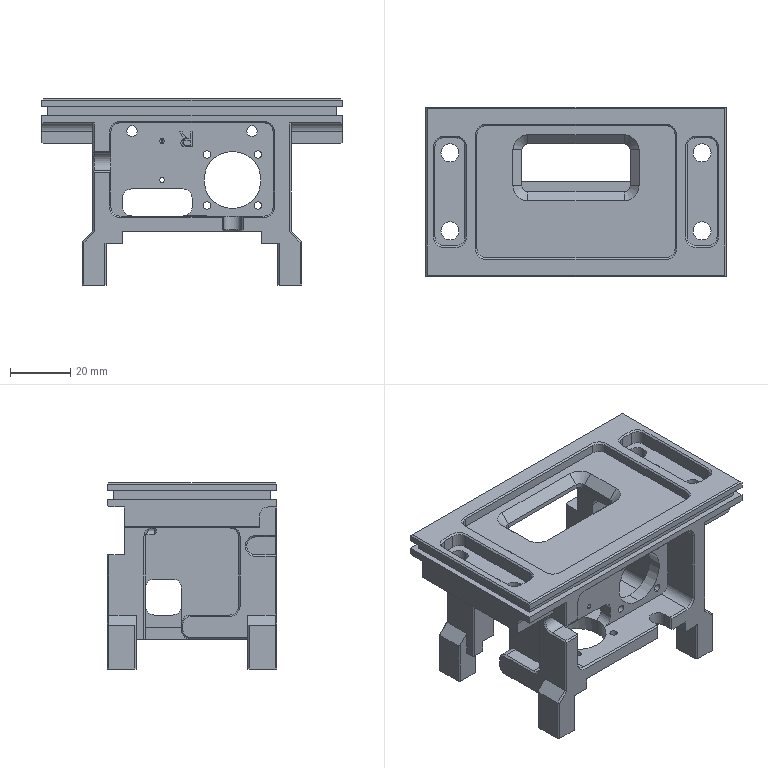NC program | Mastercam | posted with a generic post | part box 100 x 56.5 x 62 mm
Lines 30393 to 32423 of 45570, first 1872 of 2031 lines:
N6850 T11 M6
N6860 G0 G90 G17 G54 X-60. Y-16.9 A0. S8000 M3
N6870 G43 H11 Z20. M8
N6880 Z1.
N6890 G1 Z-.628 F600.
N6900 X-50. F4000.
N6910 X50.
N6920 X60.
N6930 Z-1.256 F600.
N6940 X50. F4000.
N6950 X-50.
N6960 X-60.
N6970 Z-1.883 F600.
N6980 X-50. F4000.
N6990 X50.
N7000 X60.
N7010 Z-2.511 F600.
N7020 X50. F4000.
N7030 X-50.
N7040 X-60.
N7050 Z-3.139 F600.
N7060 X-50. F4000.
N7070 X50.
N7080 X60.
N7090 Z-3.767 F600.
N7100 X50. F4000.
N7110 X-50.
N7120 X-60.
N7130 Z-4.394 F600.
N7140 X-50. F4000.
N7150 X50.
N7160 X60.
N7170 Z-5.022 F600.
N7180 X50. F4000.
N7190 X-50.
N7200 X-60.
N7210 Z-5.65 F600.
N7220 X-50. F4000.
N7230 X50.
N7240 X60.
N7250 G0 Z20.
N7260 Y-13.1
N7270 Z1.
N7280 G1 Z-.628 F600.
N7290 X50. F4000.
N7300 X-50.
N7310 X-60.
N7320 Z-1.256 F600.
N7330 X-50. F4000.
N7340 X50.
N7350 X60.
N7360 Z-1.883 F600.
N7370 X50. F4000.
N7380 X-50.
N7390 X-60.
N7400 Z-2.511 F600.
N7410 X-50. F4000.
N7420 X50.
N7430 X60.
N7440 Z-3.139 F600.
N7450 X50. F4000.
N7460 X-50.
N7470 X-60.
N7480 Z-3.767 F600.
N7490 X-50. F4000.
N7500 X50.
N7510 X60.
N7520 Z-4.394 F600.
N7530 X50. F4000.
N7540 X-50.
N7550 X-60.
N7560 Z-5.022 F600.
N7570 X-50. F4000.
N7580 X50.
N7590 X60.
N7600 Z-5.65 F600.
N7610 X50. F4000.
N7620 X-50.
N7630 X-60.
N7640 G0 Z20.
N7650 M5
N7660 G91 G28 Z0. M9
N7670 A0.
N7680 M01
N7690 T12 M6
N7700 G0 G90 G17 G54 X-60. Y-17. A0. S8000 M3
N7710 G43 H12 Z20. M8
N7720 Z-4.75
N7730 G1 Z-5.75 F600.
N7740 X-50. F1000.
N7750 X50.
N7760 X60.
N7770 G0 Z20.
N7780 Y-13.
N7790 Z-4.75
N7800 G1 Z-5.75 F600.
N7810 X50. F1000.
N7820 X-50.
N7830 X-60.
N7840 G0 Z20.
N7850 M5
N7860 G91 G28 Z0. M9
N7870 A0.
N7880 M01
N7890 T11 M6
N7900 G0 G90 G17 G54 X-2.228 Y-1.165 A0. S8000 M3
N7910 G43 H11 Z20. M8
N7920 Z1.
N7930 G1 Z.325 F600.
N7940 G3 X-7.628 Y-6.565 Z.073 I0. J-5.4 F4000.
N7950 X-2.228 Y-11.965 Z-.18 I5.4 J0.
N7960 X3.172 Y-6.565 Z-.432 I0. J5.4
N7970 X-2.228 Y-1.165 Z-.685 I-5.4 J0.
N7980 G1 X-3.035
N7990 Y-2.835
N8000 X0.
N8010 X3.035
N8020 Y-1.165
N8030 X-2.228
N8040 G2 X-2.953 Y-.582 I0. J.743
N8050 G1 X-3.73 Y2.941
N8060 G3 X-4.455 Y3.523 I-.725 J-.16
N8070 G1 X-7.723
N8080 Y-7.523
N8090 X0.
N8100 X7.723
N8110 Y3.523
N8120 X-4.455
N8130 G2 X-5.18 Y4.106 I0. J.743
N8140 G1 X-5.957 Y7.629
N8150 G3 X-6.683 Y8.212 I-.726 J-.16
N8160 G1 X-12.412
N8170 Y-12.212
N8180 X0.
N8190 X12.412
N8200 Y8.212
N8210 X-6.683
N8220 G2 X-7.408 Y8.794 I0. J.742
N8230 G1 X-8.185 Y12.317
N8240 G3 X-8.91 Y12.9 I-.725 J-.159
N8250 G1 X-16.188
N8260 X-17.087 Y12.887
N8270 X-17.1 Y12.656
N8280 Y-16.898
N8290 X-17.099 Y-16.9
N8300 X0.
N8310 X17.099
N8320 X17.1 Y12.656
N8330 X17.087 Y12.887
N8340 X16.959 Y12.898
N8350 X16.188 Y12.9
N8360 X-8.91
N8370 G0 Z20.
N8380 X-2.228 Y-1.165
N8390 Z.315
N8400 G1 Z-.36 F600.
N8410 G3 X-7.628 Y-6.565 Z-.612 I0. J-5.4 F4000.
N8420 X-2.228 Y-11.965 Z-.865 I5.4 J0.
N8430 X3.172 Y-6.565 Z-1.117 I0. J5.4
N8440 X-2.228 Y-1.165 Z-1.369 I-5.4 J0.
N8450 G1 X-3.035
N8460 Y-2.835
N8470 X0.
N8480 X3.035
N8490 Y-1.165
N8500 X-2.228
N8510 G2 X-2.953 Y-.582 I0. J.743
N8520 G1 X-3.73 Y2.941
N8530 G3 X-4.455 Y3.523 I-.725 J-.16
N8540 G1 X-7.723
N8550 Y-7.523
N8560 X0.
N8570 X7.723
N8580 Y3.523
N8590 X-4.455
N8600 G2 X-5.18 Y4.106 I0. J.743
N8610 G1 X-5.957 Y7.629
N8620 G3 X-6.683 Y8.212 I-.726 J-.16
N8630 G1 X-12.412
N8640 Y-12.212
N8650 X0.
N8660 X12.412
N8670 Y8.212
N8680 X-6.683
N8690 G2 X-7.408 Y8.794 I0. J.742
N8700 G1 X-8.185 Y12.317
N8710 G3 X-8.91 Y12.9 I-.725 J-.159
N8720 G1 X-16.188
N8730 X-17.087 Y12.887
N8740 X-17.1 Y12.656
N8750 Y-16.898
N8760 X-17.099 Y-16.9
N8770 X0.
N8780 X17.099
N8790 X17.1 Y12.656
N8800 X17.087 Y12.887
N8810 X16.959 Y12.898
N8820 X16.188 Y12.9
N8830 X-8.91
N8840 G0 Z20.
N8850 X-2.228 Y-1.165
N8860 Z-.369
N8870 G1 Z-1.044 F600.
N8880 G3 X-7.628 Y-6.565 Z-1.297 I0. J-5.4 F4000.
N8890 X-2.228 Y-11.965 Z-1.549 I5.4 J0.
N8900 X3.172 Y-6.565 Z-1.802 I0. J5.4
N8910 X-2.228 Y-1.165 Z-2.054 I-5.4 J0.
N8920 G1 X-3.035
N8930 Y-2.835
N8940 X0.
N8950 X3.035
N8960 Y-1.165
N8970 X-2.228
N8980 G2 X-2.953 Y-.582 I0. J.743
N8990 G1 X-3.73 Y2.941
N9000 G3 X-4.455 Y3.523 I-.725 J-.16
N9010 G1 X-7.723
N9020 Y-7.523
N9030 X0.
N9040 X7.723
N9050 Y3.523
N9060 X-4.455
N9070 G2 X-5.18 Y4.106 I0. J.743
N9080 G1 X-5.957 Y7.629
N9090 G3 X-6.683 Y8.212 I-.726 J-.16
N9100 G1 X-12.412
N9110 Y-12.212
N9120 X0.
N9130 X12.412
N9140 Y8.212
N9150 X-6.683
N9160 G2 X-7.408 Y8.794 I0. J.742
N9170 G1 X-8.185 Y12.317
N9180 G3 X-8.91 Y12.9 I-.725 J-.159
N9190 G1 X-16.188
N9200 X-17.087 Y12.887
N9210 X-17.1 Y12.656
N9220 Y-16.898
N9230 X-17.099 Y-16.9
N9240 X0.
N9250 X17.099
N9260 X17.1 Y12.656
N9270 X17.087 Y12.887
N9280 X16.959 Y12.898
N9290 X16.188 Y12.9
N9300 X-8.91
N9310 G0 Z20.
N9320 X-2.228 Y-1.165
N9330 Z-1.054
N9340 G1 Z-1.729 F600.
N9350 G3 X-7.628 Y-6.565 Z-1.982 I0. J-5.4 F4000.
N9360 X-2.228 Y-11.965 Z-2.234 I5.4 J0.
N9370 X3.172 Y-6.565 Z-2.486 I0. J5.4
N9380 X-2.228 Y-1.165 Z-2.739 I-5.4 J0.
N9390 G1 X-3.035
N9400 Y-2.835
N9410 X0.
N9420 X3.035
N9430 Y-1.165
N9440 X-2.228
N9450 G2 X-2.953 Y-.582 I0. J.743
N9460 G1 X-3.73 Y2.941
N9470 G3 X-4.455 Y3.523 I-.725 J-.16
N9480 G1 X-7.723
N9490 Y-7.523
N9500 X0.
N9510 X7.723
N9520 Y3.523
N9530 X-4.455
N9540 G2 X-5.18 Y4.106 I0. J.743
N9550 G1 X-5.957 Y7.629
N9560 G3 X-6.683 Y8.212 I-.726 J-.16
N9570 G1 X-12.412
N9580 Y-12.212
N9590 X0.
N9600 X12.412
N9610 Y8.212
N9620 X-6.683
N9630 G2 X-7.408 Y8.794 I0. J.742
N9640 G1 X-8.185 Y12.317
N9650 G3 X-8.91 Y12.9 I-.725 J-.159
N9660 G1 X-16.188
N9670 X-17.087 Y12.887
N9680 X-17.1 Y12.656
N9690 Y-16.898
N9700 X-17.099 Y-16.9
N9710 X0.
N9720 X17.099
N9730 X17.1 Y12.656
N9740 X17.087 Y12.887
N9750 X16.959 Y12.898
N9760 X16.188 Y12.9
N9770 X-8.91
N9780 G0 Z20.
N9790 X-2.228 Y-1.165
N9800 Z-1.739
N9810 G1 Z-2.414 F600.
N9820 G3 X-7.628 Y-6.565 Z-2.666 I0. J-5.4 F4000.
N9830 X-2.228 Y-11.965 Z-2.919 I5.4 J0.
N9840 X3.172 Y-6.565 Z-3.171 I0. J5.4
N9850 X-2.228 Y-1.165 Z-3.424 I-5.4 J0.
N9860 G1 X-3.035
N9870 Y-2.835
N9880 X0.
N9890 X3.035
N9900 Y-1.165
N9910 X-2.228
N9920 G2 X-2.953 Y-.582 I0. J.743
N9930 G1 X-3.73 Y2.941
N9940 G3 X-4.455 Y3.523 I-.725 J-.16
N9950 G1 X-7.723
N9960 Y-7.523
N9970 X0.
N9980 X7.723
N9990 Y3.523
N100 X-4.455
N110 G2 X-5.18 Y4.106 I0. J.743
N120 G1 X-5.957 Y7.629
N130 G3 X-6.683 Y8.212 I-.726 J-.16
N140 G1 X-12.412
N150 Y-12.212
N160 X0.
N170 X12.412
N180 Y8.212
N190 X-6.683
N200 G2 X-7.408 Y8.794 I0. J.742
N210 G1 X-8.185 Y12.317
N220 G3 X-8.91 Y12.9 I-.725 J-.159
N230 G1 X-16.188
N240 X-17.087 Y12.887
N250 X-17.1 Y12.656
N260 Y-16.898
N270 X-17.099 Y-16.9
N280 X0.
N290 X17.099
N300 X17.1 Y12.656
N310 X17.087 Y12.887
N320 X16.959 Y12.898
N330 X16.188 Y12.9
N340 X-8.91
N350 G0 Z20.
N360 X-2.228 Y-1.165
N370 Z-2.424
N380 G1 Z-3.099 F600.
N390 G3 X-7.628 Y-6.565 Z-3.351 I0. J-5.4 F4000.
N400 X-2.228 Y-11.965 Z-3.603 I5.4 J0.
N410 X3.172 Y-6.565 Z-3.856 I0. J5.4
N420 X-2.228 Y-1.165 Z-4.108 I-5.4 J0.
N430 G1 X-3.035
N440 Y-2.835
N450 X0.
N460 X3.035
N470 Y-1.165
N480 X-2.228
N490 G2 X-2.953 Y-.582 I0. J.743
N500 G1 X-3.73 Y2.941
N510 G3 X-4.455 Y3.523 I-.725 J-.16
N520 G1 X-7.723
N530 Y-7.523
N540 X0.
N550 X7.723
N560 Y3.523
N570 X-4.455
N580 G2 X-5.18 Y4.106 I0. J.743
N590 G1 X-5.957 Y7.629
N600 G3 X-6.683 Y8.212 I-.726 J-.16
N610 G1 X-12.412
N620 Y-12.212
N630 X0.
N640 X12.412
N650 Y8.212
N660 X-6.683
N670 G2 X-7.408 Y8.794 I0. J.742
N680 G1 X-8.185 Y12.317
N690 G3 X-8.91 Y12.9 I-.725 J-.159
N700 G1 X-16.188
N710 X-17.087 Y12.887
N720 X-17.1 Y12.656
N730 Y-16.898
N740 X-17.099 Y-16.9
N750 X0.
N760 X17.099
N770 X17.1 Y12.656
N780 X17.087 Y12.887
N790 X16.959 Y12.898
N800 X16.188 Y12.9
N810 X-8.91
N820 G0 Z20.
N830 X-2.228 Y-1.165
N840 Z-3.108
N850 G1 Z-3.783 F600.
N860 G3 X-7.628 Y-6.565 Z-4.036 I0. J-5.4 F4000.
N870 X-2.228 Y-11.965 Z-4.288 I5.4 J0.
N880 X3.172 Y-6.565 Z-4.541 I0. J5.4
N890 X-2.228 Y-1.165 Z-4.793 I-5.4 J0.
N900 G1 X-3.035
N910 Y-2.835
N920 X0.
N930 X3.035
N940 Y-1.165
N950 X-2.228
N960 G2 X-2.953 Y-.582 I0. J.743
N970 G1 X-3.73 Y2.941
N980 G3 X-4.455 Y3.523 I-.725 J-.16
N990 G1 X-7.723
N1000 Y-7.523
N1010 X0.
N1020 X7.723
N1030 Y3.523
N1040 X-4.455
N1050 G2 X-5.18 Y4.106 I0. J.743
N1060 G1 X-5.957 Y7.629
N1070 G3 X-6.683 Y8.212 I-.726 J-.16
N1080 G1 X-12.412
N1090 Y-12.212
N1100 X0.
N1110 X12.412
N1120 Y8.212
N1130 X-6.683
N1140 G2 X-7.408 Y8.794 I0. J.742
N1150 G1 X-8.185 Y12.317
N1160 G3 X-8.91 Y12.9 I-.725 J-.159
N1170 G1 X-16.188
N1180 X-17.087 Y12.887
N1190 X-17.1 Y12.656
N1200 Y-16.898
N1210 X-17.099 Y-16.9
N1220 X0.
N1230 X17.099
N1240 X17.1 Y12.656
N1250 X17.087 Y12.887
N1260 X16.959 Y12.898
N1270 X16.188 Y12.9
N1280 X-8.91
N1290 G0 Z20.
N1300 X-2.228 Y-1.165
N1310 Z-3.793
N1320 G1 Z-4.468 F600.
N1330 G3 X-7.628 Y-6.565 Z-4.72 I0. J-5.4 F4000.
N1340 X-2.228 Y-11.965 Z-4.973 I5.4 J0.
N1350 X3.172 Y-6.565 Z-5.225 I0. J5.4
N1360 X-2.228 Y-1.165 Z-5.478 I-5.4 J0.
N1370 G1 X-3.035
N1380 Y-2.835
N1390 X0.
N1400 X3.035
N1410 Y-1.165
N1420 X-2.228
N1430 G2 X-2.953 Y-.582 I0. J.743
N1440 G1 X-3.73 Y2.941
N1450 G3 X-4.455 Y3.523 I-.725 J-.16
N1460 G1 X-7.723
N1470 Y-7.523
N1480 X0.
N1490 X7.723
N1500 Y3.523
N1510 X-4.455
N1520 G2 X-5.18 Y4.106 I0. J.743
N1530 G1 X-5.957 Y7.629
N1540 G3 X-6.683 Y8.212 I-.726 J-.16
N1550 G1 X-12.412
N1560 Y-12.212
N1570 X0.
N1580 X12.412
N1590 Y8.212
N1600 X-6.683
N1610 G2 X-7.408 Y8.794 I0. J.742
N1620 G1 X-8.185 Y12.317
N1630 G3 X-8.91 Y12.9 I-.725 J-.159
N1640 G1 X-16.188
N1650 X-17.087 Y12.887
N1660 X-17.1 Y12.656
N1670 Y-16.898
N1680 X-17.099 Y-16.9
N1690 X0.
N1700 X17.099
N1710 X17.1 Y12.656
N1720 X17.087 Y12.887
N1730 X16.959 Y12.898
N1740 X16.188 Y12.9
N1750 X-8.91
N1760 G0 Z20.
N1770 X-2.228 Y-1.165
N1780 Z-4.478
N1790 G1 Z-5.153 F600.
N1800 G3 X-7.628 Y-6.565 Z-5.405 I0. J-5.4 F4000.
N1810 X-2.228 Y-11.965 Z-5.658 I5.4 J0.
N1820 X3.172 Y-6.565 Z-5.91 I0. J5.4
N1830 X-2.228 Y-1.165 Z-6.162 I-5.4 J0.
N1840 G1 X-3.035
N1850 Y-2.835
N1860 X0.
N1870 X3.035
N1880 Y-1.165
N1890 X-2.228
N1900 G2 X-2.953 Y-.582 I0. J.743
N1910 G1 X-3.73 Y2.941
N1920 G3 X-4.455 Y3.523 I-.725 J-.16
N1930 G1 X-7.723
N1940 Y-7.523
N1950 X0.
N1960 X7.723
N1970 Y3.523
N1980 X-4.455
N1990 G2 X-5.18 Y4.106 I0. J.743
N2000 G1 X-5.957 Y7.629
N2010 G3 X-6.683 Y8.212 I-.726 J-.16
N2020 G1 X-12.412
N2030 Y-12.212
N2040 X0.
N2050 X12.412
N2060 Y8.212
N2070 X-6.683
N2080 G2 X-7.408 Y8.794 I0. J.742
N2090 G1 X-8.185 Y12.317
N2100 G3 X-8.91 Y12.9 I-.725 J-.159
N2110 G1 X-16.188
N2120 X-17.087 Y12.887
N2130 X-17.1 Y12.656
N2140 Y-16.898
N2150 X-17.099 Y-16.9
N2160 X0.
N2170 X17.099
N2180 X17.1 Y12.656
N2190 X17.087 Y12.887
N2200 X16.959 Y12.898
N2210 X16.188 Y12.9
N2220 X-8.91
N2230 G0 Z20.
N2240 X-2.228 Y-1.165
N2250 Z-5.162
N2260 G1 Z-5.838 F600.
N2270 G3 X-7.628 Y-6.565 Z-6.09 I0. J-5.4 F4000.
N2280 X-2.228 Y-11.965 Z-6.342 I5.4 J0.
N2290 X3.172 Y-6.565 Z-6.595 I0. J5.4
N2300 X-2.228 Y-1.165 Z-6.847 I-5.4 J0.
N2310 G1 X-3.035
N2320 Y-2.835
N2330 X0.
N2340 X3.035
N2350 Y-1.165
N2360 X-2.228
N2370 G2 X-2.953 Y-.582 I0. J.743
N2380 G1 X-3.73 Y2.941
N2390 G3 X-4.455 Y3.523 I-.725 J-.16
N2400 G1 X-7.723
N2410 Y-7.523
N2420 X0.
N2430 X7.723
N2440 Y3.523
N2450 X-4.455
N2460 G2 X-5.18 Y4.106 I0. J.743
N2470 G1 X-5.957 Y7.629
N2480 G3 X-6.683 Y8.212 I-.726 J-.16
N2490 G1 X-12.412
N2500 Y-12.212
N2510 X0.
N2520 X12.412
N2530 Y8.212
N2540 X-6.683
N2550 G2 X-7.408 Y8.794 I0. J.742
N2560 G1 X-8.185 Y12.317
N2570 G3 X-8.91 Y12.9 I-.725 J-.159
N2580 G1 X-16.188
N2590 X-17.087 Y12.887
N2600 X-17.1 Y12.656
N2610 Y-16.898
N2620 X-17.099 Y-16.9
N2630 X0.
N2640 X17.099
N2650 X17.1 Y12.656
N2660 X17.087 Y12.887
N2670 X16.959 Y12.898
N2680 X16.188 Y12.9
N2690 X-8.91
N2700 G0 Z20.
N2710 X-2.228 Y-1.165
N2720 Z-5.847
N2730 G1 Z-6.522 F600.
N2740 G3 X-7.628 Y-6.565 Z-6.775 I0. J-5.4 F4000.
N2750 X-2.228 Y-11.965 Z-7.027 I5.4 J0.
N2760 X3.172 Y-6.565 Z-7.28 I0. J5.4
N2770 X-2.228 Y-1.165 Z-7.532 I-5.4 J0.
N2780 G1 X-3.035
N2790 Y-2.835
N2800 X0.
N2810 X3.035
N2820 Y-1.165
N2830 X-2.228
N2840 G2 X-2.953 Y-.582 I0. J.743
N2850 G1 X-3.73 Y2.941
N2860 G3 X-4.455 Y3.523 I-.725 J-.16
N2870 G1 X-7.723
N2880 Y-7.523
N2890 X0.
N2900 X7.723
N2910 Y3.523
N2920 X-4.455
N2930 G2 X-5.18 Y4.106 I0. J.743
N2940 G1 X-5.957 Y7.629
N2950 G3 X-6.683 Y8.212 I-.726 J-.16
N2960 G1 X-12.412
N2970 Y-12.212
N2980 X0.
N2990 X12.412
N3000 Y8.212
N3010 X-6.683
N3020 G2 X-7.408 Y8.794 I0. J.742
N3030 G1 X-8.185 Y12.317
N3040 G3 X-8.91 Y12.9 I-.725 J-.159
N3050 G1 X-16.188
N3060 X-17.087 Y12.887
N3070 X-17.1 Y12.656
N3080 Y-16.898
N3090 X-17.099 Y-16.9
N3100 X0.
N3110 X17.099
N3120 X17.1 Y12.656
N3130 X17.087 Y12.887
N3140 X16.959 Y12.898
N3150 X16.188 Y12.9
N3160 X-8.91
N3170 G0 Z20.
N3180 X-2.228 Y-1.165
N3190 Z-6.532
N3200 G1 Z-7.207 F600.
N3210 G3 X-7.628 Y-6.565 Z-7.459 I0. J-5.4 F4000.
N3220 X-2.228 Y-11.965 Z-7.712 I5.4 J0.
N3230 X3.172 Y-6.565 Z-7.964 I0. J5.4
N3240 X-2.228 Y-1.165 Z-8.217 I-5.4 J0.
N3250 G1 X-3.035
N3260 Y-2.835
N3270 X0.
N3280 X3.035
N3290 Y-1.165
N3300 X-2.228
N3310 G2 X-2.953 Y-.582 I0. J.743
N3320 G1 X-3.73 Y2.941
N3330 G3 X-4.455 Y3.523 I-.725 J-.16
N3340 G1 X-7.723
N3350 Y-7.523
N3360 X0.
N3370 X7.723
N3380 Y3.523
N3390 X-4.455
N3400 G2 X-5.18 Y4.106 I0. J.743
N3410 G1 X-5.957 Y7.629
N3420 G3 X-6.683 Y8.212 I-.726 J-.16
N3430 G1 X-12.412
N3440 Y-12.212
N3450 X0.
N3460 X12.412
N3470 Y8.212
N3480 X-6.683
N3490 G2 X-7.408 Y8.794 I0. J.742
N3500 G1 X-8.185 Y12.317
N3510 G3 X-8.91 Y12.9 I-.725 J-.159
N3520 G1 X-16.188
N3530 X-17.087 Y12.887
N3540 X-17.1 Y12.656
N3550 Y-16.898
N3560 X-17.099 Y-16.9
N3570 X0.
N3580 X17.099
N3590 X17.1 Y12.656
N3600 X17.087 Y12.887
N3610 X16.959 Y12.898
N3620 X16.188 Y12.9
N3630 X-8.91
N3640 G0 Z20.
N3650 X-2.228 Y-1.165
N3660 Z-7.217
N3670 G1 Z-7.892 F600.
N3680 G3 X-7.628 Y-6.565 Z-8.144 I0. J-5.4 F4000.
N3690 X-2.228 Y-11.965 Z-8.397 I5.4 J0.
N3700 X3.172 Y-6.565 Z-8.649 I0. J5.4
N3710 X-2.228 Y-1.165 Z-8.901 I-5.4 J0.
N3720 G1 X-3.035
N3730 Y-2.835
N3740 X0.
N3750 X3.035
N3760 Y-1.165
N3770 X-2.228
N3780 G2 X-2.953 Y-.582 I0. J.743
N3790 G1 X-3.73 Y2.941
N3800 G3 X-4.455 Y3.523 I-.725 J-.16
N3810 G1 X-7.723
N3820 Y-7.523
N3830 X0.
N3840 X7.723
N3850 Y3.523
N3860 X-4.455
N3870 G2 X-5.18 Y4.106 I0. J.743
N3880 G1 X-5.957 Y7.629
N3890 G3 X-6.683 Y8.212 I-.726 J-.16
N3900 G1 X-12.412
N3910 Y-12.212
N3920 X0.
N3930 X12.412
N3940 Y8.212
N3950 X-6.683
N3960 G2 X-7.408 Y8.794 I0. J.742
N3970 G1 X-8.185 Y12.317
N3980 G3 X-8.91 Y12.9 I-.725 J-.159
N3990 G1 X-16.188
N4000 X-17.087 Y12.887
N4010 X-17.1 Y12.656
N4020 Y-16.898
N4030 X-17.099 Y-16.9
N4040 X0.
N4050 X17.099
N4060 X17.1 Y12.656
N4070 X17.087 Y12.887
N4080 X16.959 Y12.898
N4090 X16.188 Y12.9
N4100 X-8.91
N4110 G0 Z20.
N4120 X-2.228 Y-1.165
N4130 Z-7.901
N4140 G1 Z-8.576 F600.
N4150 G3 X-7.628 Y-6.565 Z-8.829 I0. J-5.4 F4000.
N4160 X-2.228 Y-11.965 Z-9.081 I5.4 J0.
N4170 X3.172 Y-6.565 Z-9.334 I0. J5.4
N4180 X-2.228 Y-1.165 Z-9.586 I-5.4 J0.
N4190 G1 X-3.035
N4200 Y-2.835
N4210 X0.
N4220 X3.035
N4230 Y-1.165
N4240 X-2.228
N4250 G2 X-2.953 Y-.582 I0. J.743
N4260 G1 X-3.73 Y2.941
N4270 G3 X-4.455 Y3.523 I-.725 J-.16
N4280 G1 X-7.723
N4290 Y-7.523
N4300 X0.
N4310 X7.723
N4320 Y3.523
N4330 X-4.455
N4340 G2 X-5.18 Y4.106 I0. J.743
N4350 G1 X-5.957 Y7.629
N4360 G3 X-6.683 Y8.212 I-.726 J-.16
N4370 G1 X-12.412
N4380 Y-12.212
N4390 X0.
N4400 X12.412
N4410 Y8.212
N4420 X-6.683
N4430 G2 X-7.408 Y8.794 I0. J.742
N4440 G1 X-8.185 Y12.317
N4450 G3 X-8.91 Y12.9 I-.725 J-.159
N4460 G1 X-16.188
N4470 X-17.087 Y12.887
N4480 X-17.1 Y12.656
N4490 Y-16.898
N4500 X-17.099 Y-16.9
N4510 X0.
N4520 X17.099
N4530 X17.1 Y12.656
N4540 X17.087 Y12.887
N4550 X16.959 Y12.898
N4560 X16.188 Y12.9
N4570 X-8.91
N4580 G0 Z20.
N4590 X-2.228 Y-1.165
N4600 Z-8.586
N4610 G1 Z-9.261 F600.
N4620 G3 X-7.628 Y-6.565 Z-9.514 I0. J-5.4 F4000.
N4630 X-2.228 Y-11.965 Z-9.766 I5.4 J0.
N4640 X3.172 Y-6.565 Z-10.018 I0. J5.4
N4650 X-2.228 Y-1.165 Z-10.271 I-5.4 J0.
N4660 G1 X-3.035
N4670 Y-2.835
N4680 X0.
N4690 X3.035
N4700 Y-1.165
N4710 X-2.228
N4720 G2 X-2.953 Y-.582 I0. J.743
N4730 G1 X-3.73 Y2.941
N4740 G3 X-4.455 Y3.523 I-.725 J-.16
N4750 G1 X-7.723
N4760 Y-7.523
N4770 X0.
N4780 X7.723
N4790 Y3.523
N4800 X-4.455
N4810 G2 X-5.18 Y4.106 I0. J.743
N4820 G1 X-5.957 Y7.629
N4830 G3 X-6.683 Y8.212 I-.726 J-.16
N4840 G1 X-12.412
N4850 Y-12.212
N4860 X0.
N4870 X12.412
N4880 Y8.212
N4890 X-6.683
N4900 G2 X-7.408 Y8.794 I0. J.742
N4910 G1 X-8.185 Y12.317
N4920 G3 X-8.91 Y12.9 I-.725 J-.159
N4930 G1 X-16.188
N4940 X-17.087 Y12.887
N4950 X-17.1 Y12.656
N4960 Y-16.898
N4970 X-17.099 Y-16.9
N4980 X0.
N4990 X17.099
N5000 X17.1 Y12.656
N5010 X17.087 Y12.887
N5020 X16.959 Y12.898
N5030 X16.188 Y12.9
N5040 X-8.91
N5050 G0 Z20.
N5060 X-2.228 Y-1.165
N5070 Z-9.271
N5080 G1 Z-9.946 F600.
N5090 G3 X-7.628 Y-6.565 Z-10.198 I0. J-5.4 F4000.
N5100 X-2.228 Y-11.965 Z-10.451 I5.4 J0.
N5110 X3.172 Y-6.565 Z-10.703 I0. J5.4
N5120 X-2.228 Y-1.165 Z-10.956 I-5.4 J0.
N5130 G1 X-3.035
N5140 Y-2.835
N5150 X0.
N5160 X3.035
N5170 Y-1.165
N5180 X-2.228
N5190 G2 X-2.953 Y-.582 I0. J.743
N5200 G1 X-3.73 Y2.941
N5210 G3 X-4.455 Y3.523 I-.725 J-.16
N5220 G1 X-7.723
N5230 Y-7.523
N5240 X0.
N5250 X7.723
N5260 Y3.523
N5270 X-4.455
N5280 G2 X-5.18 Y4.106 I0. J.743
N5290 G1 X-5.957 Y7.629
N5300 G3 X-6.683 Y8.212 I-.726 J-.16
N5310 G1 X-12.412
N5320 Y-12.212
N5330 X0.
N5340 X12.412
N5350 Y8.212
N5360 X-6.683
N5370 G2 X-7.408 Y8.794 I0. J.742
N5380 G1 X-8.185 Y12.317
N5390 G3 X-8.91 Y12.9 I-.725 J-.159
N5400 G1 X-16.188
N5410 X-17.087 Y12.887
N5420 X-17.1 Y12.656
N5430 Y-16.898
N5440 X-17.099 Y-16.9
N5450 X0.
N5460 X17.099
N5470 X17.1 Y12.656
N5480 X17.087 Y12.887
N5490 X16.959 Y12.898
N5500 X16.188 Y12.9
N5510 X-8.91
N5520 G0 Z20.
N5530 X-2.228 Y-1.165
N5540 Z-9.956
N5550 G1 Z-10.631 F600.
N5560 G3 X-7.628 Y-6.565 Z-10.883 I0. J-5.4 F4000.
N5570 X-2.228 Y-11.965 Z-11.135 I5.4 J0.
N5580 X3.172 Y-6.565 Z-11.388 I0. J5.4
N5590 X-2.228 Y-1.165 Z-11.64 I-5.4 J0.
N5600 G1 X-3.035
N5610 Y-2.835
N5620 X0.
N5630 X3.035
N5640 Y-1.165
N5650 X-2.228
N5660 G2 X-2.953 Y-.582 I0. J.743
N5670 G1 X-3.73 Y2.941
N5680 G3 X-4.455 Y3.523 I-.725 J-.16
N5690 G1 X-7.723
N5700 Y-7.523
N5710 X0.
N5720 X7.723
N5730 Y3.523
N5740 X-4.455
N5750 G2 X-5.18 Y4.106 I0. J.743
N5760 G1 X-5.957 Y7.629
N5770 G3 X-6.683 Y8.212 I-.726 J-.16
N5780 G1 X-12.412
N5790 Y-12.212
N5800 X0.
N5810 X12.412
N5820 Y8.212
N5830 X-6.683
N5840 G2 X-7.408 Y8.794 I0. J.742
N5850 G1 X-8.185 Y12.317
N5860 G3 X-8.91 Y12.9 I-.725 J-.159
N5870 G1 X-16.188
N5880 X-17.087 Y12.887
N5890 X-17.1 Y12.656
N5900 Y-16.898
N5910 X-17.099 Y-16.9
N5920 X0.
N5930 X17.099
N5940 X17.1 Y12.656
N5950 X17.087 Y12.887
N5960 X16.959 Y12.898
N5970 X16.188 Y12.9
N5980 X-8.91
N5990 G0 Z20.
N6000 X-2.228 Y-1.165
N6010 Z-10.64
N6020 G1 Z-11.315 F600.
N6030 G3 X-7.628 Y-6.565 Z-11.568 I0. J-5.4 F4000.
N6040 X-2.228 Y-11.965 Z-11.82 I5.4 J0.
N6050 X3.172 Y-6.565 Z-12.073 I0. J5.4
N6060 X-2.228 Y-1.165 Z-12.325 I-5.4 J0.
N6070 G1 X-3.035
N6080 Y-2.835
N6090 X0.
N6100 X3.035
N6110 Y-1.165
N6120 X-2.228
N6130 G2 X-2.953 Y-.582 I0. J.743
N6140 G1 X-3.73 Y2.941
N6150 G3 X-4.455 Y3.523 I-.725 J-.16
N6160 G1 X-7.723
N6170 Y-7.523
N6180 X0.
N6190 X7.723
N6200 Y3.523
N6210 X-4.455
N6220 G2 X-5.18 Y4.106 I0. J.743
N6230 G1 X-5.957 Y7.629
N6240 G3 X-6.683 Y8.212 I-.726 J-.16
N6250 G1 X-12.412
N6260 Y-12.212
N6270 X0.
N6280 X12.412
N6290 Y8.212
N6300 X-6.683
N6310 G2 X-7.408 Y8.794 I0. J.742
N6320 G1 X-8.185 Y12.317
N6330 G3 X-8.91 Y12.9 I-.725 J-.159
N6340 G1 X-16.188
N6350 X-17.087 Y12.887
N6360 X-17.1 Y12.656
N6370 Y-16.898
N6380 X-17.099 Y-16.9
N6390 X0.
N6400 X17.099
N6410 X17.1 Y12.656
N6420 X17.087 Y12.887
N6430 X16.959 Y12.898
N6440 X16.188 Y12.9
N6450 X-8.91
N6460 G0 Z20.
N6470 X-2.228 Y-1.165
N6480 Z-11.325
N6490 G1 Z-12. F600.
N6500 G3 X-7.628 Y-6.565 Z-12.252 I0. J-5.4 F4000.
N6510 X-2.228 Y-11.965 Z-12.505 I5.4 J0.
N6520 X3.172 Y-6.565 Z-12.757 I0. J5.4
N6530 X-2.228 Y-1.165 Z-13.01 I-5.4 J0.
N6540 G1 X-3.035
N6550 Y-2.835
N6560 X0.
N6570 X3.035
N6580 Y-1.165
N6590 X-2.228
N6600 G2 X-2.953 Y-.582 I0. J.743
N6610 G1 X-3.73 Y2.941
N6620 G3 X-4.455 Y3.523 I-.725 J-.16
N6630 G1 X-7.723
N6640 Y-7.523
N6650 X0.
N6660 X7.723
N6670 Y3.523
N6680 X-4.455
N6690 G2 X-5.18 Y4.106 I0. J.743
N6700 G1 X-5.957 Y7.629
N6710 G3 X-6.683 Y8.212 I-.726 J-.16
N6720 G1 X-12.412
N6730 Y-12.212
N6740 X0.
N6750 X12.412
N6760 Y8.212
N6770 X-6.683
N6780 G2 X-7.408 Y8.794 I0. J.742
N6790 G1 X-8.185 Y12.317
N6800 G3 X-8.91 Y12.9 I-.725 J-.159
N6810 G1 X-16.188
N6820 X-17.087 Y12.887
N6830 X-17.1 Y12.656
N6840 Y-16.898
N6850 X-17.099 Y-16.9
N6860 X0.
N6870 X17.099
N6880 X17.1 Y12.656
N6890 X17.087 Y12.887
N6900 X16.959 Y12.898
N6910 X16.188 Y12.9
N6920 X-8.91
N6930 G0 Z20.
N6940 X-2.228 Y-1.165
N6950 Z-12.01
N6960 G1 Z-12.685 F600.
N6970 G3 X-7.628 Y-6.565 Z-12.937 I0. J-5.4 F4000.
N6980 X-2.228 Y-11.965 Z-13.19 I5.4 J0.
N6990 X3.172 Y-6.565 Z-13.442 I0. J5.4
N7000 X-2.228 Y-1.165 Z-13.694 I-5.4 J0.
N7010 G1 X-3.035
N7020 Y-2.835
N7030 X0.
N7040 X3.035
N7050 Y-1.165
N7060 X-2.228
N7070 G2 X-2.953 Y-.582 I0. J.743
N7080 G1 X-3.73 Y2.941
N7090 G3 X-4.455 Y3.523 I-.725 J-.16
N7100 G1 X-7.723
N7110 Y-7.523
N7120 X0.
N7130 X7.723
N7140 Y3.523
N7150 X-4.455
N7160 G2 X-5.18 Y4.106 I0. J.743
N7170 G1 X-5.957 Y7.629
N7180 G3 X-6.683 Y8.212 I-.726 J-.16
N7190 G1 X-12.412
N7200 Y-12.212
N7210 X0.
N7220 X12.412
N7230 Y8.212
N7240 X-6.683
N7250 G2 X-7.408 Y8.794 I0. J.742
N7260 G1 X-8.185 Y12.317
N7270 G3 X-8.91 Y12.9 I-.725 J-.159
N7280 G1 X-16.188
N7290 X-17.087 Y12.887
N7300 X-17.1 Y12.656
N7310 Y-16.898
N7320 X-17.099 Y-16.9
N7330 X0.
N7340 X17.099
N7350 X17.1 Y12.656
N7360 X17.087 Y12.887
N7370 X16.959 Y12.898
N7380 X16.188 Y12.9
N7390 X-8.91
N7400 G0 Z20.
N7410 X-2.228 Y-1.165
N7420 Z-12.694
N7430 G1 Z-13.369 F600.
N7440 G3 X-7.628 Y-6.565 Z-13.622 I0. J-5.4 F4000.
N7450 X-2.228 Y-11.965 Z-13.874 I5.4 J0.
N7460 X3.172 Y-6.565 Z-14.127 I0. J5.4
N7470 X-2.228 Y-1.165 Z-14.379 I-5.4 J0.
N7480 G1 X-3.035
N7490 Y-2.835
N7500 X0.
N7510 X3.035
N7520 Y-1.165
N7530 X-2.228
N7540 G2 X-2.953 Y-.582 I0. J.743
N7550 G1 X-3.73 Y2.941
N7560 G3 X-4.455 Y3.523 I-.725 J-.16
N7570 G1 X-7.723
N7580 Y-7.523
N7590 X0.
N7600 X7.723
N7610 Y3.523
N7620 X-4.455
N7630 G2 X-5.18 Y4.106 I0. J.743
N7640 G1 X-5.957 Y7.629
N7650 G3 X-6.683 Y8.212 I-.726 J-.16
N7660 G1 X-12.412
N7670 Y-12.212
N7680 X0.
N7690 X12.412
N7700 Y8.212
N7710 X-6.683
N7720 G2 X-7.408 Y8.794 I0. J.742
N7730 G1 X-8.185 Y12.317
N7740 G3 X-8.91 Y12.9 I-.725 J-.159
N7750 G1 X-16.188
N7760 X-17.087 Y12.887
N7770 X-17.1 Y12.656
N7780 Y-16.898
N7790 X-17.099 Y-16.9
N7800 X0.
N7810 X17.099
N7820 X17.1 Y12.656
N7830 X17.087 Y12.887
N7840 X16.959 Y12.898
N7850 X16.188 Y12.9
N7860 X-8.91
N7870 G0 Z20.
N7880 X-2.228 Y-1.165
N7890 Z-13.379
N7900 G1 Z-14.054 F600.
N7910 G3 X-7.628 Y-6.565 Z-14.307 I0. J-5.4 F4000.
N7920 X-2.228 Y-11.965 Z-14.559 I5.4 J0.
N7930 X3.172 Y-6.565 Z-14.811 I0. J5.4
N7940 X-2.228 Y-1.165 Z-15.064 I-5.4 J0.
N7950 G1 X-3.035
N7960 Y-2.835
N7970 X0.
N7980 X3.035
N7990 Y-1.165
N8000 X-2.228
N8010 G2 X-2.953 Y-.582 I0. J.743
N8020 G1 X-3.73 Y2.941
N8030 G3 X-4.455 Y3.523 I-.725 J-.16
N8040 G1 X-7.723
N8050 Y-7.523
N8060 X0.
N8070 X7.723
N8080 Y3.523
N8090 X-4.455
N8100 G2 X-5.18 Y4.106 I0. J.743
N8110 G1 X-5.957 Y7.629
N8120 G3 X-6.683 Y8.212 I-.726 J-.16
N8130 G1 X-12.412
N8140 Y-12.212
N8150 X0.
N8160 X12.412
N8170 Y8.212
N8180 X-6.683
N8190 G2 X-7.408 Y8.794 I0. J.742
N8200 G1 X-8.185 Y12.317
N8210 G3 X-8.91 Y12.9 I-.725 J-.159
N8220 G1 X-16.188
N8230 X-17.087 Y12.887
N8240 X-17.1 Y12.656
N8250 Y-16.898
N8260 X-17.099 Y-16.9
N8270 X0.
N8280 X17.099
N8290 X17.1 Y12.656
N8300 X17.087 Y12.887
N8310 X16.959 Y12.898
N8320 X16.188 Y12.9
N8330 X-8.91
N8340 G0 Z20.
N8350 X-2.228 Y-1.165
N8360 Z-14.064
N8370 G1 Z-14.739 F600.
N8380 G3 X-7.628 Y-6.565 Z-14.991 I0. J-5.4 F4000.
N8390 X-2.228 Y-11.965 Z-15.244 I5.4 J0.
N8400 X3.172 Y-6.565 Z-15.496 I0. J5.4
N8410 X-2.228 Y-1.165 Z-15.749 I-5.4 J0.
N8420 G1 X-3.035
N8430 Y-2.835
N8440 X0.
N8450 X3.035
N8460 Y-1.165
N8470 X-2.228
N8480 G2 X-2.953 Y-.582 I0. J.743
N8490 G1 X-3.73 Y2.941
N8500 G3 X-4.455 Y3.523 I-.725 J-.16
N8510 G1 X-7.723
N8520 Y-7.523
N8530 X0.
N8540 X7.723
N8550 Y3.523
N8560 X-4.455
N8570 G2 X-5.18 Y4.106 I0. J.743
N8580 G1 X-5.957 Y7.629
N8590 G3 X-6.683 Y8.212 I-.726 J-.16
N8600 G1 X-12.412
N8610 Y-12.212
N8620 X0.
N8630 X12.412
N8640 Y8.212
N8650 X-6.683
N8660 G2 X-7.408 Y8.794 I0. J.742
N8670 G1 X-8.185 Y12.317
N8680 G3 X-8.91 Y12.9 I-.725 J-.159
N8690 G1 X-16.188
N8700 X-17.087 Y12.887
N8710 X-17.1 Y12.656
N8720 Y-16.898
N8730 X-17.099 Y-16.9
N8740 X0.
N8750 X17.099
N8760 X17.1 Y12.656
N8770 X17.087 Y12.887
N8780 X16.959 Y12.898
N8790 X16.188 Y12.9
N8800 X-8.91
N8810 G0 Z20.
N8820 X-2.228 Y-1.165
N8830 Z-14.749
N8840 G1 Z-15.424 F600.
N8850 G3 X-7.628 Y-6.565 Z-15.676 I0. J-5.4 F4000.
N8860 X-2.228 Y-11.965 Z-15.928 I5.4 J0.
N8870 X3.172 Y-6.565 Z-16.181 I0. J5.4
N8880 X-2.228 Y-1.165 Z-16.433 I-5.4 J0.
N8890 G1 X-3.035
N8900 Y-2.835
N8910 X0.
N8920 X3.035
N8930 Y-1.165
N8940 X-2.228
N8950 G2 X-2.953 Y-.582 I0. J.743
N8960 G1 X-3.73 Y2.941
N8970 G3 X-4.455 Y3.523 I-.725 J-.16
N8980 G1 X-7.723
N8990 Y-7.523
N9000 X0.
N9010 X7.723
N9020 Y3.523
N9030 X-4.455
N9040 G2 X-5.18 Y4.106 I0. J.743
N9050 G1 X-5.957 Y7.629
N9060 G3 X-6.683 Y8.212 I-.726 J-.16
N9070 G1 X-12.412
N9080 Y-12.212
N9090 X0.
N9100 X12.412
N9110 Y8.212
N9120 X-6.683
N9130 G2 X-7.408 Y8.794 I0. J.742
N9140 G1 X-8.185 Y12.317
N9150 G3 X-8.91 Y12.9 I-.725 J-.159
N9160 G1 X-16.188
N9170 X-17.087 Y12.887
N9180 X-17.1 Y12.656
N9190 Y-16.898
N9200 X-17.099 Y-16.9
N9210 X0.
N9220 X17.099
N9230 X17.1 Y12.656
N9240 X17.087 Y12.887
N9250 X16.959 Y12.898
N9260 X16.188 Y12.9
N9270 X-8.91
N9280 G0 Z20.
N9290 X-2.228 Y-1.165
N9300 Z-15.433
N9310 G1 Z-16.108 F600.
N9320 G3 X-7.628 Y-6.565 Z-16.361 I0. J-5.4 F4000.
N9330 X-2.228 Y-11.965 Z-16.613 I5.4 J0.
N9340 X3.172 Y-6.565 Z-16.866 I0. J5.4
N9350 X-2.228 Y-1.165 Z-17.118 I-5.4 J0.
N9360 G1 X-3.035
N9370 Y-2.835
N9380 X0.
N9390 X3.035
N9400 Y-1.165
N9410 X-2.228
N9420 G2 X-2.953 Y-.582 I0. J.743
N9430 G1 X-3.73 Y2.941
N9440 G3 X-4.455 Y3.523 I-.725 J-.16
N9450 G1 X-7.723
N9460 Y-7.523
N9470 X0.
N9480 X7.723
N9490 Y3.523
N9500 X-4.455
N9510 G2 X-5.18 Y4.106 I0. J.743
N9520 G1 X-5.957 Y7.629
N9530 G3 X-6.683 Y8.212 I-.726 J-.16
N9540 G1 X-12.412
N9550 Y-12.212
N9560 X0.
N9570 X12.412
N9580 Y8.212
N9590 X-6.683
N9600 G2 X-7.408 Y8.794 I0. J.742
N9610 G1 X-8.185 Y12.317
N9620 G3 X-8.91 Y12.9 I-.725 J-.159
N9630 G1 X-16.188
N9640 X-17.087 Y12.887
N9650 X-17.1 Y12.656
N9660 Y-16.898
N9670 X-17.099 Y-16.9
N9680 X0.
N9690 X17.099
N9700 X17.1 Y12.656
N9710 X17.087 Y12.887
N9720 X16.959 Y12.898
N9730 X16.188 Y12.9
N9740 X-8.91
N9750 G0 Z20.
N9760 X-2.228 Y-1.165
N9770 Z-16.118
N9780 G1 Z-16.793 F600.
N9790 G3 X-7.628 Y-6.565 Z-17.045 I0. J-5.4 F4000.
N9800 X-2.228 Y-11.965 Z-17.298 I5.4 J0.
N9810 X3.172 Y-6.565 Z-17.55 I0. J5.4
N9820 X-2.228 Y-1.165 Z-17.803 I-5.4 J0.
N9830 G1 X-3.035
N9840 Y-2.835
N9850 X0.
N9860 X3.035
N9870 Y-1.165
N9880 X-2.228
N9890 G2 X-2.953 Y-.582 I0. J.743
N9900 G1 X-3.73 Y2.941
N9910 G3 X-4.455 Y3.523 I-.725 J-.16
N9920 G1 X-7.723
N9930 Y-7.523
N9940 X0.
N9950 X7.723
N9960 Y3.523
N9970 X-4.455
N9980 G2 X-5.18 Y4.106 I0. J.743
N9990 G1 X-5.957 Y7.629
N100 G3 X-6.683 Y8.212 I-.726 J-.16
N110 G1 X-12.412
N120 Y-12.212
N130 X0.
N140 X12.412
N150 Y8.212
N160 X-6.683
N170 G2 X-7.408 Y8.794 I0. J.742
N180 G1 X-8.185 Y12.317
N190 G3 X-8.91 Y12.9 I-.725 J-.159
N200 G1 X-16.188
N210 X-17.087 Y12.887
N220 X-17.1 Y12.656
N230 Y-16.898
N240 X-17.099 Y-16.9
N250 X0.
N260 X17.099
N270 X17.1 Y12.656
N280 X17.087 Y12.887
N290 X16.959 Y12.898
N300 X16.188 Y12.9
N310 X-8.91
N320 G0 Z20.
N330 X-2.228 Y-1.165
N340 Z-16.803
N350 G1 Z-17.478 F600.
N360 G3 X-7.628 Y-6.565 Z-17.73 I0. J-5.4 F4000.
N370 X-2.228 Y-11.965 Z-17.983 I5.4 J0.
N380 X3.172 Y-6.565 Z-18.235 I0. J5.4
N390 X-2.228 Y-1.165 Z-18.488 I-5.4 J0.
N400 G1 X-3.035
N410 Y-2.835
N420 X0.
N430 X3.035
N440 Y-1.165
N450 X-2.228
N460 G2 X-2.953 Y-.582 I0. J.743
N470 G1 X-3.73 Y2.941
N480 G3 X-4.455 Y3.523 I-.725 J-.16
N490 G1 X-7.723
N500 Y-7.523
N510 X0.
N520 X7.723
N530 Y3.523
N540 X-4.455
N550 G2 X-5.18 Y4.106 I0. J.743
N560 G1 X-5.957 Y7.629
N570 G3 X-6.683 Y8.212 I-.726 J-.16
N580 G1 X-12.412
N590 Y-12.212
N600 X0.
N610 X12.412
N620 Y8.212
N630 X-6.683
N640 G2 X-7.408 Y8.794 I0. J.742
N650 G1 X-8.185 Y12.317
N660 G3 X-8.91 Y12.9 I-.725 J-.159
N670 G1 X-16.188
N680 X-17.087 Y12.887
N690 X-17.1 Y12.656
N700 Y-16.898
N710 X-17.099 Y-16.9
N720 X0.
N730 X17.099
N740 X17.1 Y12.656
N750 X17.087 Y12.887
N760 X16.959 Y12.898
N770 X16.188 Y12.9
N780 X-8.91
N790 G0 Z20.
N800 X-2.228 Y-1.165
N810 Z-17.488
N820 G1 Z-18.163 F600.
N830 G3 X-7.628 Y-6.565 Z-18.415 I0. J-5.4 F4000.
N840 X-2.228 Y-11.965 Z-18.667 I5.4 J0.
N850 X3.172 Y-6.565 Z-18.92 I0. J5.4
N860 X-2.228 Y-1.165 Z-19.172 I-5.4 J0.
N870 G1 X-3.035
N880 Y-2.835
N890 X0.
N900 X3.035
N910 Y-1.165
N920 X-2.228
N930 G2 X-2.953 Y-.582 I0. J.743
N940 G1 X-3.73 Y2.941
N950 G3 X-4.455 Y3.523 I-.725 J-.16
N960 G1 X-7.723
N970 Y-7.523
N980 X0.
N990 X7.723
N1000 Y3.523
N1010 X-4.455
N1020 G2 X-5.18 Y4.106 I0. J.743
N1030 G1 X-5.957 Y7.629
N1040 G3 X-6.683 Y8.212 I-.726 J-.16
N1050 G1 X-12.412
N1060 Y-12.212
N1070 X0.
N1080 X12.412
N1090 Y8.212
N1100 X-6.683
N1110 G2 X-7.408 Y8.794 I0. J.742
N1120 G1 X-8.185 Y12.317
N1130 G3 X-8.91 Y12.9 I-.725 J-.159
N1140 G1 X-16.188
N1150 X-17.087 Y12.887
N1160 X-17.1 Y12.656
N1170 Y-16.898
N1180 X-17.099 Y-16.9
N1190 X0.
N1200 X17.099
N1210 X17.1 Y12.656
N1220 X17.087 Y12.887
N1230 X16.959 Y12.898
N1240 X16.188 Y12.9
N1250 X-8.91
N1260 G0 Z20.
N1270 X-2.228 Y-1.165
N1280 Z-18.172
N1290 G1 Z-18.847 F600.
N1300 G3 X-7.628 Y-6.565 Z-19.1 I0. J-5.4 F4000.
N1310 X-2.228 Y-11.965 Z-19.352 I5.4 J0.
N1320 X3.172 Y-6.565 Z-19.605 I0. J5.4
N1330 X-2.228 Y-1.165 Z-19.857 I-5.4 J0.
N1340 G1 X-3.035
N1350 Y-2.835
N1360 X0.
N1370 X3.035
N1380 Y-1.165
N1390 X-2.228
N1400 G2 X-2.953 Y-.582 I0. J.743
N1410 G1 X-3.73 Y2.941
N1420 G3 X-4.455 Y3.523 I-.725 J-.16
N1430 G1 X-7.723
N1440 Y-7.523
N1450 X0.
N1460 X7.723
N1470 Y3.523
N1480 X-4.455
N1490 G2 X-5.18 Y4.106 I0. J.743
N1500 G1 X-5.957 Y7.629
N1510 G3 X-6.683 Y8.212 I-.726 J-.16
N1520 G1 X-12.412
N1530 Y-12.212
N1540 X0.
N1550 X12.412
N1560 Y8.212
N1570 X-6.683
N1580 G2 X-7.408 Y8.794 I0. J.742
N1590 G1 X-8.185 Y12.317
N1600 G3 X-8.91 Y12.9 I-.725 J-.159
N1610 G1 X-16.188
N1620 X-17.087 Y12.887
N1630 X-17.1 Y12.656
N1640 Y-16.898
N1650 X-17.099 Y-16.9
N1660 X0.
N1670 X17.099
N1680 X17.1 Y12.656
N1690 X17.087 Y12.887
N1700 X16.959 Y12.898
N1710 X16.188 Y12.9
N1720 X-8.91
N1730 G0 Z20.
N1740 X-2.228 Y-1.165
N1750 Z-18.857
N1760 G1 Z-19.532 F600.
N1770 G3 X-7.628 Y-6.565 Z-19.784 I0. J-5.4 F4000.
N1780 X-2.228 Y-11.965 Z-20.037 I5.4 J0.
N1790 X3.172 Y-6.565 Z-20.289 I0. J5.4
N1800 X-2.228 Y-1.165 Z-20.542 I-5.4 J0.
N1810 G1 X-3.035
N1820 Y-2.835
N1830 X0.
N1840 X3.035
N1850 Y-1.165
N1860 X-2.228
N1870 G2 X-2.953 Y-.582 I0. J.743
N1880 G1 X-3.73 Y2.941
N1890 G3 X-4.455 Y3.523 I-.725 J-.16
N1900 G1 X-7.723
N1910 Y-7.523
N1920 X0.
N1930 X7.723
N1940 Y3.523
N1950 X-4.455
N1960 G2 X-5.18 Y4.106 I0. J.743
N1970 G1 X-5.957 Y7.629
N1980 G3 X-6.683 Y8.212 I-.726 J-.16
N1990 G1 X-12.412
N2000 Y-12.212
N2010 X0.
N2020 X12.412
N2030 Y8.212
N2040 X-6.683
N2050 G2 X-7.408 Y8.794 I0. J.742
N2060 G1 X-8.185 Y12.317
N2070 G3 X-8.91 Y12.9 I-.725 J-.159
N2080 G1 X-16.188
N2090 X-17.087 Y12.887
N2100 X-17.1 Y12.656
N2110 Y-16.898
N2120 X-17.099 Y-16.9
N2130 X0.
N2140 X17.099
N2150 X17.1 Y12.656
N2160 X17.087 Y12.887
N2170 X16.959 Y12.898
N2180 X16.188 Y12.9
N2190 X-8.91
N2200 G0 Z20.
N2210 X-2.228 Y-1.165
N2220 Z-19.542
N2230 G1 Z-20.217 F600.
N2240 G3 X-7.628 Y-6.565 Z-20.469 I0. J-5.4 F4000.
N2250 X-2.228 Y-11.965 Z-20.722 I5.4 J0.
N2260 X3.172 Y-6.565 Z-20.974 I0. J5.4
N2270 X-2.228 Y-1.165 Z-21.226 I-5.4 J0.
N2280 G1 X-3.035
N2290 Y-2.835
N2300 X0.
N2310 X3.035
N2320 Y-1.165
N2330 X-2.228
N2340 G2 X-2.953 Y-.582 I0. J.743
N2350 G1 X-3.73 Y2.941
N2360 G3 X-4.455 Y3.523 I-.725 J-.16
N2370 G1 X-7.723
N2380 Y-7.523
N2390 X0.
N2400 X7.723
N2410 Y3.523
N2420 X-4.455
N2430 G2 X-5.18 Y4.106 I0. J.743
N2440 G1 X-5.957 Y7.629
N2450 G3 X-6.683 Y8.212 I-.726 J-.16
N2460 G1 X-12.412
N2470 Y-12.212
N2480 X0.
N2490 X12.412
N2500 Y8.212
N2510 X-6.683
N2520 G2 X-7.408 Y8.794 I0. J.742
N2530 G1 X-8.185 Y12.317
N2540 G3 X-8.91 Y12.9 I-.725 J-.159
N2550 G1 X-16.188
N2560 X-17.087 Y12.887
N2570 X-17.1 Y12.656
N2580 Y-16.898
N2590 X-17.099 Y-16.9
N2600 X0.
N2610 X17.099
N2620 X17.1 Y12.656
N2630 X17.087 Y12.887
N2640 X16.959 Y12.898
N2650 X16.188 Y12.9
N2660 X-8.91
N2670 G0 Z20.
N2680 X-2.228 Y-1.165
N2690 Z-20.226
N2700 G1 Z-20.901 F600.
N2710 G3 X-7.628 Y-6.565 Z-21.154 I0. J-5.4 F4000.
N2720 X-2.228 Y-11.965 Z-21.406 I5.4 J0.
N2730 X3.172 Y-6.565 Z-21.659 I0. J5.4
N2740 X-2.228 Y-1.165 Z-21.911 I-5.4 J0.
N2750 G1 X-3.035
N2760 Y-2.835
N2770 X0.
N2780 X3.035
N2790 Y-1.165
N2800 X-2.228
N2810 G2 X-2.953 Y-.582 I0. J.743
N2820 G1 X-3.73 Y2.941
N2830 G3 X-4.455 Y3.523 I-.725 J-.16
N2840 G1 X-7.723
N2850 Y-7.523
N2860 X0.
N2870 X7.723
N2880 Y3.523
N2890 X-4.455
N2900 G2 X-5.18 Y4.106 I0. J.743
N2910 G1 X-5.957 Y7.629
N2920 G3 X-6.683 Y8.212 I-.726 J-.16
N2930 G1 X-12.412
N2940 Y-12.212
N2950 X0.
N2960 X12.412
N2970 Y8.212
N2980 X-6.683
N2990 G2 X-7.408 Y8.794 I0. J.742
N3000 G1 X-8.185 Y12.317
N3010 G3 X-8.91 Y12.9 I-.725 J-.159
N3020 G1 X-16.188
N3030 X-17.087 Y12.887
N3040 X-17.1 Y12.656
N3050 Y-16.898
N3060 X-17.099 Y-16.9
N3070 X0.
N3080 X17.099
N3090 X17.1 Y12.656
N3100 X17.087 Y12.887
N3110 X16.959 Y12.898
N3120 X16.188 Y12.9
N3130 X-8.91
N3140 G0 Z20.
N3150 X-2.228 Y-1.165
N3160 Z-20.911
N3170 G1 Z-21.586 F600.
N3180 G3 X-7.628 Y-6.565 Z-21.839 I0. J-5.4 F4000.
N3190 X-2.228 Y-11.965 Z-22.091 I5.4 J0.
N3200 X3.172 Y-6.565 Z-22.343 I0. J5.4
N3210 X-2.228 Y-1.165 Z-22.596 I-5.4 J0.
N3220 G1 X-3.035
N3230 Y-2.835
N3240 X0.
N3250 X3.035
N3260 Y-1.165
N3270 X-2.228
N3280 G2 X-2.953 Y-.582 I0. J.743
N3290 G1 X-3.73 Y2.941
N3300 G3 X-4.455 Y3.523 I-.725 J-.16
N3310 G1 X-7.723
N3320 Y-7.523
N3330 X0.
N3340 X7.723
N3350 Y3.523
N3360 X-4.455
N3370 G2 X-5.18 Y4.106 I0. J.743
N3380 G1 X-5.957 Y7.629
N3390 G3 X-6.683 Y8.212 I-.726 J-.16
N3400 G1 X-12.412
N3410 Y-12.212
N3420 X0.
N3430 X12.412
N3440 Y8.212
N3450 X-6.683
N3460 G2 X-7.408 Y8.794 I0. J.742
N3470 G1 X-8.185 Y12.317
N3480 G3 X-8.91 Y12.9 I-.725 J-.159
N3490 G1 X-16.188
N3500 X-17.087 Y12.887
N3510 X-17.1 Y12.656
N3520 Y-16.898
N3530 X-17.099 Y-16.9
N3540 X0.
N3550 X17.099
N3560 X17.1 Y12.656
N3570 X17.087 Y12.887
N3580 X16.959 Y12.898
N3590 X16.188 Y12.9
N3600 X-8.91
N3610 G0 Z20.
N3620 X-2.228 Y-1.165
N3630 Z-21.596
N3640 G1 Z-22.271 F600.
N3650 G3 X-7.628 Y-6.565 Z-22.523 I0. J-5.4 F4000.
N3660 X-2.228 Y-11.965 Z-22.776 I5.4 J0.
N3670 X3.172 Y-6.565 Z-23.028 I0. J5.4
N3680 X-2.228 Y-1.165 Z-23.281 I-5.4 J0.
N3690 G1 X-3.035
N3700 Y-2.835
N3710 X0.
N3720 X3.035
N3730 Y-1.165
N3740 X-2.228
N3750 G2 X-2.953 Y-.582 I0. J.743
N3760 G1 X-3.73 Y2.941
N3770 G3 X-4.455 Y3.523 I-.725 J-.16
N3780 G1 X-7.723
N3790 Y-7.523
N3800 X0.
N3810 X7.723
N3820 Y3.523
N3830 X-4.455
N3840 G2 X-5.18 Y4.106 I0. J.743
N3850 G1 X-5.957 Y7.629
N3860 G3 X-6.683 Y8.212 I-.726 J-.16
N3870 G1 X-12.412
N3880 Y-12.212
N3890 X0.
N3900 X12.412
N3910 Y8.212
N3920 X-6.683
N3930 G2 X-7.408 Y8.794 I0. J.742
N3940 G1 X-8.185 Y12.317
N3950 G3 X-8.91 Y12.9 I-.725 J-.159
N3960 G1 X-16.188
N3970 X-17.087 Y12.887
N3980 X-17.1 Y12.656
N3990 Y-16.898
N4000 X-17.099 Y-16.9
N4010 X0.
N4020 X17.099
N4030 X17.1 Y12.656
N4040 X17.087 Y12.887
N4050 X16.959 Y12.898
N4060 X16.188 Y12.9
N4070 X-8.91
N4080 G0 Z20.
N4090 X-2.228 Y-1.165
N4100 Z-22.281
N4110 G1 Z-22.956 F600.
N4120 G3 X-7.628 Y-6.565 Z-23.208 I0. J-5.4 F4000.
N4130 X-2.228 Y-11.965 Z-23.46 I5.4 J0.
N4140 X3.172 Y-6.565 Z-23.713 I0. J5.4
N4150 X-2.228 Y-1.165 Z-23.965 I-5.4 J0.
N4160 G1 X-3.035
N4170 Y-2.835
N4180 X0.
N4190 X3.035
N4200 Y-1.165
N4210 X-2.228
N4220 G2 X-2.953 Y-.582 I0. J.743
N4230 G1 X-3.73 Y2.941
N4240 G3 X-4.455 Y3.523 I-.725 J-.16
N4250 G1 X-7.723
N4260 Y-7.523
N4270 X0.
N4280 X7.723
N4290 Y3.523
N4300 X-4.455
N4310 G2 X-5.18 Y4.106 I0. J.743
N4320 G1 X-5.957 Y7.629
N4330 G3 X-6.683 Y8.212 I-.726 J-.16
N4340 G1 X-12.412
N4350 Y-12.212
N4360 X0.
N4370 X12.412
N4380 Y8.212
N4390 X-6.683
N4400 G2 X-7.408 Y8.794 I0. J.742
N4410 G1 X-8.185 Y12.317
N4420 G3 X-8.91 Y12.9 I-.725 J-.159
N4430 G1 X-16.188
N4440 X-17.087 Y12.887
N4450 X-17.1 Y12.656
N4460 Y-16.898
N4470 X-17.099 Y-16.9
N4480 X0.
N4490 X17.099
N4500 X17.1 Y12.656
N4510 X17.087 Y12.887
N4520 X16.959 Y12.898
N4530 X16.188 Y12.9
N4540 X-8.91
N4550 G0 Z20.
N4560 X-2.228 Y-1.165
N4570 Z-22.965
N4580 G1 Z-23.64 F600.
N4590 G3 X-7.628 Y-6.565 Z-23.893 I0. J-5.4 F4000.
N4600 X-2.228 Y-11.965 Z-24.145 I5.4 J0.
N4610 X3.172 Y-6.565 Z-24.398 I0. J5.4
N4620 X-2.228 Y-1.165 Z-24.65 I-5.4 J0.
N4630 G1 X-3.035
N4640 Y-2.835
N4650 X0.
N4660 X3.035
N4670 Y-1.165
N4680 X-2.228
N4690 G2 X-2.953 Y-.582 I0. J.743
N4700 G1 X-3.73 Y2.941
N4710 G3 X-4.455 Y3.523 I-.725 J-.16
N4720 G1 X-7.723
N4730 Y-7.523
N4740 X0.
N4750 X7.723
N4760 Y3.523
N4770 X-4.455
N4780 G2 X-5.18 Y4.106 I0. J.743
N4790 G1 X-5.957 Y7.629
N4800 G3 X-6.683 Y8.212 I-.726 J-.16
N4810 G1 X-12.412
N4820 Y-12.212
N4830 X0.
N4840 X12.412
N4850 Y8.212
N4860 X-6.683
N4870 G2 X-7.408 Y8.794 I0. J.742
N4880 G1 X-8.185 Y12.317
N4890 G3 X-8.91 Y12.9 I-.725 J-.159
N4900 G1 X-16.188
N4910 X-17.087 Y12.887
N4920 X-17.1 Y12.656
N4930 Y-16.898
N4940 X-17.099 Y-16.9
N4950 X0.
N4960 X17.099
N4970 X17.1 Y12.656
N4980 X17.087 Y12.887
N4990 X16.959 Y12.898
N5000 X16.188 Y12.9
N5010 X-8.91
N5020 G0 Z20.
N5030 M5
N5040 G91 G28 Z0. M9
N5050 A0.
N5060 M01
N5070 T12 M6
N5080 G0 G90 G17 G54 X1.697 Y11.8 A0. S8000 M3
N5090 G43 H12 Z20. M8
N5100 Z1.
N5110 G1 Z-12.375 F600.
N5120 X.849 Y12.649 F1000.
N5130 G3 X0. Y13. I-.849 J-.849
N5140 G1 X-17.2
N5150 Y-7.
N5160 Y-17.
N5170 X17.2
N5180 Y-7.
N5190 Y13.
N5200 X0.
N5210 X-.5
N5220 G3 X-1.349 Y12.649 I0. J-1.2
N5230 G1 X-2.197 Y11.8
N5240 X1.697
N5250 Z-24.75 F600.
N5260 X.849 Y12.649 F1000.
N5270 G3 X0. Y13. I-.849 J-.849
N5280 G1 X-17.2
N5290 Y-7.
N5300 Y-17.
N5310 X17.2
N5320 Y-7.
N5330 Y13.
N5340 X0.
N5350 X-.5
N5360 G3 X-1.349 Y12.649 I0. J-1.2
N5370 G1 X-2.197 Y11.8
N5380 G0 Z20.
N5390 M5
N5400 G91 G28 Z0. M9
N5410 A0.
N5420 M01
N5430 T11 M6
N5440 G0 G90 G17 G54 X12.1 Y-3.1 A0. S8000 M3
N5450 G43 H11 Z20. M8
N5460 Z-23.75
N5470 G1 Z-24.75 F600.
N5480 X-12.1 Z-25.007 F2000.
N5490 Y-11.9 Z-25.1
N5500 X12.1 Z-25.357
N5510 Y-3.1 Z-25.45
N5520 X-12.1 Z-25.707
N5530 Y-11.9 Z-25.8
N5540 X12.1 Z-26.057
N5550 Y-3.1 Z-26.15
N5560 X-12.1 Z-26.407
N5570 Y-11.9 Z-26.5
N5580 X12.1 Z-26.757
N5590 Y-3.1 Z-26.85
N5600 X-12.1 Z-27.107
N5610 Y-11.9 Z-27.2
N5620 X12.1 Z-27.457
N5630 Y-3.1 Z-27.55
N5640 X-12.1 Z-27.807
N5650 Y-11.9 Z-27.9
N5660 X12.1 Z-28.157
N5670 Y-3.1 Z-28.25
N5680 X-12.1 Z-28.507
N5690 Y-11.9 Z-28.6
N5700 X12.1 Z-28.857
N5710 Y-3.1 Z-28.95
N5720 X-12.1 Z-29.207
N5730 Y-11.9 Z-29.3
N5740 X12.1 Z-29.557
N5750 Y-3.1 Z-29.65
N5760 X-11.471 Z-29.9